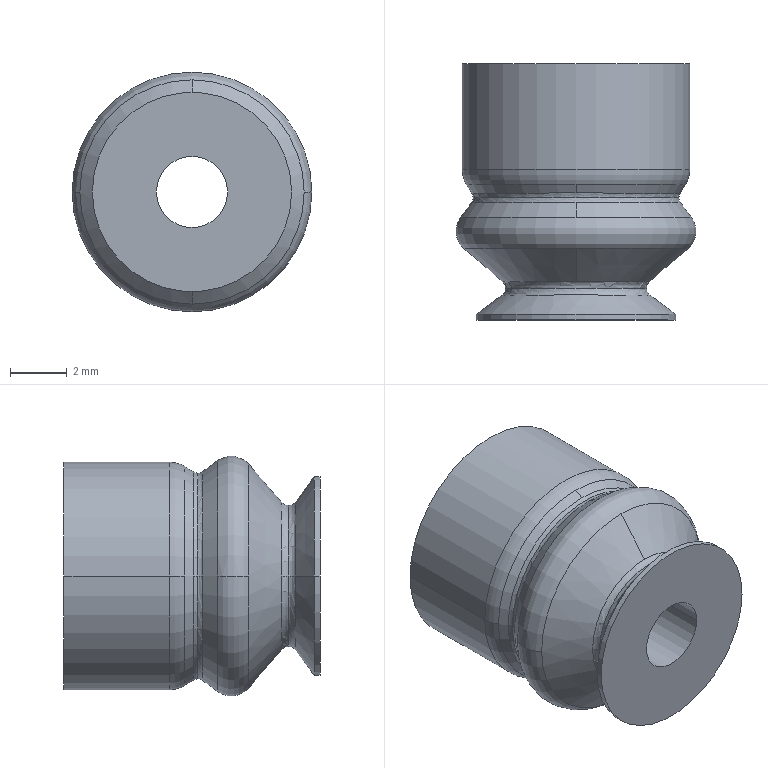Part | SolidWorks | features BaseBody 1 | 1 solid | 28 faces | box 8.435 x 9 x 8.435 mm | volume 355.359 mm3 | torus 12 | cone 8 | cylinder 6 | plane 2 | commonest cylinder face diameters 2.5 x2 7 x2 8 x2
STEP:
#1=CARTESIAN_POINT('',(-3.662,4.459,0.));
#2=VERTEX_POINT('',#1);
#3=CARTESIAN_POINT('',(-3.616,4.3,0.));
#4=VERTEX_POINT('',#3);
#5=CARTESIAN_POINT('',(-3.916,4.3,0.));
#6=DIRECTION('',(0.,0.,-1.));
#7=DIRECTION('',(0.,1.,0.));
#8=AXIS2_PLACEMENT_3D('',#5,#6,#7);
#9=CIRCLE('',#8,0.3);
#10=EDGE_CURVE('',#2,#4,#9,.T.);
#11=ORIENTED_EDGE('',*,*,#10,.T.);
#12=CARTESIAN_POINT('',(3.616,4.3,0.));
#13=VERTEX_POINT('',#12);
#14=CARTESIAN_POINT('',(0.,4.3,0.));
#15=DIRECTION('',(0.,1.,0.));
#16=DIRECTION('',(-1.,0.,0.));
#17=AXIS2_PLACEMENT_3D('',#14,#15,#16);
#18=CIRCLE('',#17,3.616);
#19=EDGE_CURVE('',#4,#13,#18,.T.);
#20=ORIENTED_EDGE('',*,*,#19,.T.);
#21=CARTESIAN_POINT('',(3.662,4.459,0.));
#22=VERTEX_POINT('',#21);
#23=CARTESIAN_POINT('',(3.916,4.3,0.));
#24=DIRECTION('',(0.,0.,1.));
#25=DIRECTION('',(1.,0.,0.));
#26=AXIS2_PLACEMENT_3D('',#23,#24,#25);
#27=CIRCLE('',#26,0.3);
#28=EDGE_CURVE('',#22,#13,#27,.T.);
#29=ORIENTED_EDGE('',*,*,#28,.F.);
#30=CARTESIAN_POINT('',(0.,4.459,3.662));
#31=VERTEX_POINT('',#30);
#32=CARTESIAN_POINT('',(0.,4.459,0.));
#33=DIRECTION('',(0.,1.,0.));
#34=DIRECTION('',(1.,0.,0.));
#35=AXIS2_PLACEMENT_3D('',#32,#33,#34);
#36=CIRCLE('',#35,3.662);
#37=EDGE_CURVE('',#31,#22,#36,.T.);
#38=ORIENTED_EDGE('',*,*,#37,.F.);
#39=CARTESIAN_POINT('',(0.,4.459,0.));
#40=DIRECTION('',(0.,1.,0.));
#41=DIRECTION('',(1.,0.,0.));
#42=AXIS2_PLACEMENT_3D('',#39,#40,#41);
#43=CIRCLE('',#42,3.662);
#44=EDGE_CURVE('',#2,#31,#43,.T.);
#45=ORIENTED_EDGE('',*,*,#44,.F.);
#46=EDGE_LOOP('',(#11,#20,#29,#38,#45));
#47=FACE_OUTER_BOUND('',#46,.T.);
#48=CARTESIAN_POINT('',(0.,4.3,0.));
#49=DIRECTION('',(0.,1.,0.));
#50=DIRECTION('',(-1.,0.,0.));
#51=AXIS2_PLACEMENT_3D('',#48,#49,#50);
#52=TOROIDAL_SURFACE('',#51,3.916,0.3);
#53=ADVANCED_FACE('',(#47),#52,.F.);
#54=CARTESIAN_POINT('',(-2.582,1.344,0.));
#55=VERTEX_POINT('',#54);
#56=CARTESIAN_POINT('',(-2.478,1.116,0.));
#57=VERTEX_POINT('',#56);
#58=CARTESIAN_POINT('',(-2.778,1.116,0.));
#59=DIRECTION('',(0.,0.,-1.));
#60=DIRECTION('',(-1.,0.,0.));
#61=AXIS2_PLACEMENT_3D('',#58,#59,#60);
#62=CIRCLE('',#61,0.3);
#63=EDGE_CURVE('',#55,#57,#62,.T.);
#64=ORIENTED_EDGE('',*,*,#63,.T.);
#65=CARTESIAN_POINT('',(2.478,1.116,0.));
#66=VERTEX_POINT('',#65);
#67=CARTESIAN_POINT('',(0.,1.116,0.));
#68=DIRECTION('',(0.,1.,0.));
#69=DIRECTION('',(-1.,0.,0.));
#70=AXIS2_PLACEMENT_3D('',#67,#68,#69);
#71=CIRCLE('',#70,2.478);
#72=EDGE_CURVE('',#57,#66,#71,.T.);
#73=ORIENTED_EDGE('',*,*,#72,.T.);
#74=CARTESIAN_POINT('',(2.582,1.344,0.));
#75=VERTEX_POINT('',#74);
#76=CARTESIAN_POINT('',(2.778,1.116,0.));
#77=DIRECTION('',(0.,0.,1.));
#78=DIRECTION('',(1.,0.,0.));
#79=AXIS2_PLACEMENT_3D('',#76,#77,#78);
#80=CIRCLE('',#79,0.3);
#81=EDGE_CURVE('',#75,#66,#80,.T.);
#82=ORIENTED_EDGE('',*,*,#81,.F.);
#83=CARTESIAN_POINT('',(0.,1.344,2.582));
#84=VERTEX_POINT('',#83);
#85=CARTESIAN_POINT('',(0.,1.344,0.));
#86=DIRECTION('',(0.,1.,0.));
#87=DIRECTION('',(0.,0.,1.));
#88=AXIS2_PLACEMENT_3D('',#85,#86,#87);
#89=CIRCLE('',#88,2.582);
#90=EDGE_CURVE('',#84,#75,#89,.T.);
#91=ORIENTED_EDGE('',*,*,#90,.F.);
#92=CARTESIAN_POINT('',(0.,1.344,0.));
#93=DIRECTION('',(0.,1.,0.));
#94=DIRECTION('',(0.,0.,1.));
#95=AXIS2_PLACEMENT_3D('',#92,#93,#94);
#96=CIRCLE('',#95,2.582);
#97=EDGE_CURVE('',#55,#84,#96,.T.);
#98=ORIENTED_EDGE('',*,*,#97,.F.);
#99=EDGE_LOOP('',(#64,#73,#82,#91,#98));
#100=FACE_OUTER_BOUND('',#99,.T.);
#101=CARTESIAN_POINT('',(0.,1.116,0.));
#102=DIRECTION('',(0.,1.,0.));
#103=DIRECTION('',(-1.,0.,0.));
#104=AXIS2_PLACEMENT_3D('',#101,#102,#103);
#105=TOROIDAL_SURFACE('',#104,2.778,0.3);
#106=ADVANCED_FACE('',(#100),#105,.F.);
#107=ORIENTED_EDGE('',*,*,#81,.T.);
#108=CARTESIAN_POINT('',(0.,1.116,0.));
#109=DIRECTION('',(0.,1.,0.));
#110=DIRECTION('',(-1.,0.,0.));
#111=AXIS2_PLACEMENT_3D('',#108,#109,#110);
#112=CIRCLE('',#111,2.478);
#113=EDGE_CURVE('',#66,#57,#112,.T.);
#114=ORIENTED_EDGE('',*,*,#113,.T.);
#115=ORIENTED_EDGE('',*,*,#63,.F.);
#116=CARTESIAN_POINT('',(0.,1.344,-2.582));
#117=VERTEX_POINT('',#116);
#118=CARTESIAN_POINT('',(0.,1.344,0.));
#119=DIRECTION('',(0.,1.,0.));
#120=DIRECTION('',(0.,0.,1.));
#121=AXIS2_PLACEMENT_3D('',#118,#119,#120);
#122=CIRCLE('',#121,2.582);
#123=EDGE_CURVE('',#117,#55,#122,.T.);
#124=ORIENTED_EDGE('',*,*,#123,.F.);
#125=CARTESIAN_POINT('',(0.,1.344,0.));
#126=DIRECTION('',(0.,1.,0.));
#127=DIRECTION('',(0.,0.,1.));
#128=AXIS2_PLACEMENT_3D('',#125,#126,#127);
#129=CIRCLE('',#128,2.582);
#130=EDGE_CURVE('',#75,#117,#129,.T.);
#131=ORIENTED_EDGE('',*,*,#130,.F.);
#132=EDGE_LOOP('',(#107,#114,#115,#124,#131));
#133=FACE_OUTER_BOUND('',#132,.T.);
#134=CARTESIAN_POINT('',(0.,1.116,0.));
#135=DIRECTION('',(0.,1.,0.));
#136=DIRECTION('',(-1.,0.,0.));
#137=AXIS2_PLACEMENT_3D('',#134,#135,#136);
#138=TOROIDAL_SURFACE('',#137,2.778,0.3);
#139=ADVANCED_FACE('',(#133),#138,.F.);
#140=ORIENTED_EDGE('',*,*,#28,.T.);
#141=CARTESIAN_POINT('',(0.,4.3,0.));
#142=DIRECTION('',(0.,1.,0.));
#143=DIRECTION('',(-1.,0.,0.));
#144=AXIS2_PLACEMENT_3D('',#141,#142,#143);
#145=CIRCLE('',#144,3.616);
#146=EDGE_CURVE('',#13,#4,#145,.T.);
#147=ORIENTED_EDGE('',*,*,#146,.T.);
#148=ORIENTED_EDGE('',*,*,#10,.F.);
#149=CARTESIAN_POINT('',(0.,4.459,-3.662));
#150=VERTEX_POINT('',#149);
#151=CARTESIAN_POINT('',(0.,4.459,0.));
#152=DIRECTION('',(0.,1.,0.));
#153=DIRECTION('',(1.,0.,0.));
#154=AXIS2_PLACEMENT_3D('',#151,#152,#153);
#155=CIRCLE('',#154,3.662);
#156=EDGE_CURVE('',#150,#2,#155,.T.);
#157=ORIENTED_EDGE('',*,*,#156,.F.);
#158=CARTESIAN_POINT('',(0.,4.459,0.));
#159=DIRECTION('',(0.,1.,0.));
#160=DIRECTION('',(1.,0.,0.));
#161=AXIS2_PLACEMENT_3D('',#158,#159,#160);
#162=CIRCLE('',#161,3.662);
#163=EDGE_CURVE('',#22,#150,#162,.T.);
#164=ORIENTED_EDGE('',*,*,#163,.F.);
#165=EDGE_LOOP('',(#140,#147,#148,#157,#164));
#166=FACE_OUTER_BOUND('',#165,.T.);
#167=CARTESIAN_POINT('',(0.,4.3,0.));
#168=DIRECTION('',(0.,1.,0.));
#169=DIRECTION('',(-1.,0.,0.));
#170=AXIS2_PLACEMENT_3D('',#167,#168,#169);
#171=TOROIDAL_SURFACE('',#170,3.916,0.3);
#172=ADVANCED_FACE('',(#166),#171,.F.);
#173=CARTESIAN_POINT('',(0.,4.757,3.848));
#174=VERTEX_POINT('',#173);
#175=CARTESIAN_POINT('',(3.848,4.757,0.));
#176=VERTEX_POINT('',#175);
#177=CARTESIAN_POINT('',(0.,4.757,0.));
#178=DIRECTION('',(0.,1.,0.));
#179=DIRECTION('',(0.,0.,1.));
#180=AXIS2_PLACEMENT_3D('',#177,#178,#179);
#181=CIRCLE('',#180,3.848);
#182=EDGE_CURVE('',#174,#176,#181,.T.);
#183=ORIENTED_EDGE('',*,*,#182,.T.);
#184=CARTESIAN_POINT('',(4.,5.287,0.));
#185=VERTEX_POINT('',#184);
#186=CARTESIAN_POINT('',(3.,5.287,0.));
#187=DIRECTION('',(0.,0.,1.));
#188=DIRECTION('',(1.,0.,0.));
#189=AXIS2_PLACEMENT_3D('',#186,#187,#188);
#190=CIRCLE('',#189,1.);
#191=EDGE_CURVE('',#176,#185,#190,.T.);
#192=ORIENTED_EDGE('',*,*,#191,.T.);
#193=CARTESIAN_POINT('',(-4.,5.287,0.));
#194=VERTEX_POINT('',#193);
#195=CARTESIAN_POINT('',(0.,5.287,0.));
#196=DIRECTION('',(0.,1.,0.));
#197=DIRECTION('',(1.,0.,0.));
#198=AXIS2_PLACEMENT_3D('',#195,#196,#197);
#199=CIRCLE('',#198,4.);
#200=EDGE_CURVE('',#194,#185,#199,.T.);
#201=ORIENTED_EDGE('',*,*,#200,.F.);
#202=CARTESIAN_POINT('',(-3.848,4.757,0.));
#203=VERTEX_POINT('',#202);
#204=CARTESIAN_POINT('',(-3.,5.287,0.));
#205=DIRECTION('',(0.,0.,-1.));
#206=DIRECTION('',(-1.,0.,0.));
#207=AXIS2_PLACEMENT_3D('',#204,#205,#206);
#208=CIRCLE('',#207,1.);
#209=EDGE_CURVE('',#203,#194,#208,.T.);
#210=ORIENTED_EDGE('',*,*,#209,.F.);
#211=CARTESIAN_POINT('',(0.,4.757,0.));
#212=DIRECTION('',(0.,1.,0.));
#213=DIRECTION('',(0.,0.,1.));
#214=AXIS2_PLACEMENT_3D('',#211,#212,#213);
#215=CIRCLE('',#214,3.848);
#216=EDGE_CURVE('',#203,#174,#215,.T.);
#217=ORIENTED_EDGE('',*,*,#216,.T.);
#218=EDGE_LOOP('',(#183,#192,#201,#210,#217));
#219=FACE_OUTER_BOUND('',#218,.T.);
#220=CARTESIAN_POINT('',(0.,5.287,0.));
#221=DIRECTION('',(0.,1.,0.));
#222=DIRECTION('',(-1.,0.,0.));
#223=AXIS2_PLACEMENT_3D('',#220,#221,#222);
#224=TOROIDAL_SURFACE('',#223,3.,1.);
#225=ADVANCED_FACE('',(#219),#224,.T.);
#226=ORIENTED_EDGE('',*,*,#146,.F.);
#227=CARTESIAN_POINT('',(3.675,4.122,0.));
#228=VERTEX_POINT('',#227);
#229=CARTESIAN_POINT('',(3.916,4.3,0.));
#230=DIRECTION('',(0.,0.,1.));
#231=DIRECTION('',(1.,0.,0.));
#232=AXIS2_PLACEMENT_3D('',#229,#230,#231);
#233=CIRCLE('',#232,0.3);
#234=EDGE_CURVE('',#13,#228,#233,.T.);
#235=ORIENTED_EDGE('',*,*,#234,.T.);
#236=CARTESIAN_POINT('',(0.,4.122,-3.675));
#237=VERTEX_POINT('',#236);
#238=CARTESIAN_POINT('',(0.,4.122,0.));
#239=DIRECTION('',(0.,-1.,0.));
#240=DIRECTION('',(0.,0.,1.));
#241=AXIS2_PLACEMENT_3D('',#238,#239,#240);
#242=CIRCLE('',#241,3.675);
#243=EDGE_CURVE('',#237,#228,#242,.T.);
#244=ORIENTED_EDGE('',*,*,#243,.F.);
#245=CARTESIAN_POINT('',(-3.675,4.122,0.));
#246=VERTEX_POINT('',#245);
#247=CARTESIAN_POINT('',(0.,4.122,0.));
#248=DIRECTION('',(0.,-1.,0.));
#249=DIRECTION('',(0.,0.,1.));
#250=AXIS2_PLACEMENT_3D('',#247,#248,#249);
#251=CIRCLE('',#250,3.675);
#252=EDGE_CURVE('',#246,#237,#251,.T.);
#253=ORIENTED_EDGE('',*,*,#252,.F.);
#254=CARTESIAN_POINT('',(-3.916,4.3,0.));
#255=DIRECTION('',(0.,0.,-1.));
#256=DIRECTION('',(0.,1.,0.));
#257=AXIS2_PLACEMENT_3D('',#254,#255,#256);
#258=CIRCLE('',#257,0.3);
#259=EDGE_CURVE('',#4,#246,#258,.T.);
#260=ORIENTED_EDGE('',*,*,#259,.F.);
#261=EDGE_LOOP('',(#226,#235,#244,#253,#260));
#262=FACE_OUTER_BOUND('',#261,.T.);
#263=CARTESIAN_POINT('',(0.,4.3,0.));
#264=DIRECTION('',(0.,1.,0.));
#265=DIRECTION('',(-1.,0.,0.));
#266=AXIS2_PLACEMENT_3D('',#263,#264,#265);
#267=TOROIDAL_SURFACE('',#266,3.916,0.3);
#268=ADVANCED_FACE('',(#262),#267,.F.);
#269=ORIENTED_EDGE('',*,*,#113,.F.);
#270=CARTESIAN_POINT('',(2.598,0.8765,0.));
#271=VERTEX_POINT('',#270);
#272=CARTESIAN_POINT('',(2.778,1.116,0.));
#273=DIRECTION('',(0.,0.,1.));
#274=DIRECTION('',(1.,0.,0.));
#275=AXIS2_PLACEMENT_3D('',#272,#273,#274);
#276=CIRCLE('',#275,0.3);
#277=EDGE_CURVE('',#66,#271,#276,.T.);
#278=ORIENTED_EDGE('',*,*,#277,.T.);
#279=CARTESIAN_POINT('',(-2.598,0.8765,0.));
#280=VERTEX_POINT('',#279);
#281=CARTESIAN_POINT('',(0.,0.8765,0.));
#282=DIRECTION('',(0.,-1.,0.));
#283=DIRECTION('',(1.,0.,0.));
#284=AXIS2_PLACEMENT_3D('',#281,#282,#283);
#285=CIRCLE('',#284,2.598);
#286=EDGE_CURVE('',#280,#271,#285,.T.);
#287=ORIENTED_EDGE('',*,*,#286,.F.);
#288=CARTESIAN_POINT('',(-2.778,1.116,0.));
#289=DIRECTION('',(0.,0.,-1.));
#290=DIRECTION('',(-1.,0.,0.));
#291=AXIS2_PLACEMENT_3D('',#288,#289,#290);
#292=CIRCLE('',#291,0.3);
#293=EDGE_CURVE('',#57,#280,#292,.T.);
#294=ORIENTED_EDGE('',*,*,#293,.F.);
#295=EDGE_LOOP('',(#269,#278,#287,#294));
#296=FACE_OUTER_BOUND('',#295,.T.);
#297=CARTESIAN_POINT('',(0.,1.116,0.));
#298=DIRECTION('',(0.,1.,0.));
#299=DIRECTION('',(-1.,0.,0.));
#300=AXIS2_PLACEMENT_3D('',#297,#298,#299);
#301=TOROIDAL_SURFACE('',#300,2.778,0.3);
#302=ADVANCED_FACE('',(#296),#301,.F.);
#303=CARTESIAN_POINT('',(0.,2.517,3.94));
#304=VERTEX_POINT('',#303);
#305=CARTESIAN_POINT('',(3.94,2.517,0.));
#306=VERTEX_POINT('',#305);
#307=CARTESIAN_POINT('',(0.,2.517,0.));
#308=DIRECTION('',(0.,1.,0.));
#309=DIRECTION('',(0.,0.,1.));
#310=AXIS2_PLACEMENT_3D('',#307,#308,#309);
#311=CIRCLE('',#310,3.94);
#312=EDGE_CURVE('',#304,#306,#311,.T.);
#313=ORIENTED_EDGE('',*,*,#312,.T.);
#314=CARTESIAN_POINT('',(4.062,3.596,0.));
#315=VERTEX_POINT('',#314);
#316=CARTESIAN_POINT('',(3.417,3.122,0.));
#317=DIRECTION('',(0.,0.,1.));
#318=DIRECTION('',(1.,0.,0.));
#319=AXIS2_PLACEMENT_3D('',#316,#317,#318);
#320=CIRCLE('',#319,0.8);
#321=EDGE_CURVE('',#306,#315,#320,.T.);
#322=ORIENTED_EDGE('',*,*,#321,.T.);
#323=CARTESIAN_POINT('',(0.,3.596,4.062));
#324=VERTEX_POINT('',#323);
#325=CARTESIAN_POINT('',(0.,3.596,0.));
#326=DIRECTION('',(0.,1.,0.));
#327=DIRECTION('',(1.,0.,0.));
#328=AXIS2_PLACEMENT_3D('',#325,#326,#327);
#329=CIRCLE('',#328,4.062);
#330=EDGE_CURVE('',#324,#315,#329,.T.);
#331=ORIENTED_EDGE('',*,*,#330,.F.);
#332=CARTESIAN_POINT('',(-4.062,3.596,0.));
#333=VERTEX_POINT('',#332);
#334=CARTESIAN_POINT('',(0.,3.596,0.));
#335=DIRECTION('',(0.,1.,0.));
#336=DIRECTION('',(1.,0.,0.));
#337=AXIS2_PLACEMENT_3D('',#334,#335,#336);
#338=CIRCLE('',#337,4.062);
#339=EDGE_CURVE('',#333,#324,#338,.T.);
#340=ORIENTED_EDGE('',*,*,#339,.F.);
#341=CARTESIAN_POINT('',(-3.94,2.517,0.));
#342=VERTEX_POINT('',#341);
#343=CARTESIAN_POINT('',(-3.417,3.122,0.));
#344=DIRECTION('',(0.,0.,-1.));
#345=DIRECTION('',(-1.,0.,0.));
#346=AXIS2_PLACEMENT_3D('',#343,#344,#345);
#347=CIRCLE('',#346,0.8);
#348=EDGE_CURVE('',#342,#333,#347,.T.);
#349=ORIENTED_EDGE('',*,*,#348,.F.);
#350=CARTESIAN_POINT('',(0.,2.517,0.));
#351=DIRECTION('',(0.,1.,0.));
#352=DIRECTION('',(0.,0.,1.));
#353=AXIS2_PLACEMENT_3D('',#350,#351,#352);
#354=CIRCLE('',#353,3.94);
#355=EDGE_CURVE('',#342,#304,#354,.T.);
#356=ORIENTED_EDGE('',*,*,#355,.T.);
#357=EDGE_LOOP('',(#313,#322,#331,#340,#349,#356));
#358=FACE_OUTER_BOUND('',#357,.T.);
#359=CARTESIAN_POINT('',(0.,3.122,0.));
#360=DIRECTION('',(0.,1.,0.));
#361=DIRECTION('',(-1.,0.,0.));
#362=AXIS2_PLACEMENT_3D('',#359,#360,#361);
#363=TOROIDAL_SURFACE('',#362,3.417,0.8);
#364=ADVANCED_FACE('',(#358),#363,.T.);
#365=CARTESIAN_POINT('',(4.,9.,0.));
#366=VERTEX_POINT('',#365);
#367=CARTESIAN_POINT('',(-4.,9.,0.));
#368=VERTEX_POINT('',#367);
#369=CARTESIAN_POINT('',(0.,9.,0.));
#370=DIRECTION('',(0.,-1.,0.));
#371=DIRECTION('',(1.,0.,0.));
#372=AXIS2_PLACEMENT_3D('',#369,#370,#371);
#373=CIRCLE('',#372,4.);
#374=EDGE_CURVE('',#366,#368,#373,.T.);
#375=ORIENTED_EDGE('',*,*,#374,.T.);
#376=CARTESIAN_POINT('',(-4.,7.143,0.));
#377=DIRECTION('',(0.,-1.,0.));
#378=VECTOR('',#377,1000.);
#379=LINE('',#376,#378);
#380=EDGE_CURVE('',#368,#194,#379,.T.);
#381=ORIENTED_EDGE('',*,*,#380,.T.);
#382=ORIENTED_EDGE('',*,*,#200,.T.);
#383=CARTESIAN_POINT('',(4.,7.143,0.));
#384=DIRECTION('',(0.,-1.,0.));
#385=VECTOR('',#384,1000.);
#386=LINE('',#383,#385);
#387=EDGE_CURVE('',#366,#185,#386,.T.);
#388=ORIENTED_EDGE('',*,*,#387,.F.);
#389=EDGE_LOOP('',(#375,#381,#382,#388));
#390=FACE_OUTER_BOUND('',#389,.T.);
#391=CARTESIAN_POINT('',(0.,7.143,0.));
#392=DIRECTION('',(0.,-1.,0.));
#393=DIRECTION('',(1.,0.,0.));
#394=AXIS2_PLACEMENT_3D('',#391,#392,#393);
#395=CYLINDRICAL_SURFACE('',#394,4.);
#396=ADVANCED_FACE('',(#390),#395,.T.);
#397=CARTESIAN_POINT('',(-1.25,9.,0.));
#398=VERTEX_POINT('',#397);
#399=CARTESIAN_POINT('',(1.25,9.,0.));
#400=VERTEX_POINT('',#399);
#401=CARTESIAN_POINT('',(0.,9.,0.));
#402=DIRECTION('',(0.,-1.,0.));
#403=DIRECTION('',(1.,0.,0.));
#404=AXIS2_PLACEMENT_3D('',#401,#402,#403);
#405=CIRCLE('',#404,1.25);
#406=EDGE_CURVE('',#398,#400,#405,.T.);
#407=ORIENTED_EDGE('',*,*,#406,.F.);
#408=CARTESIAN_POINT('',(-1.25,0.,0.));
#409=VERTEX_POINT('',#408);
#410=CARTESIAN_POINT('',(-1.25,4.5,0.));
#411=DIRECTION('',(0.,-1.,0.));
#412=VECTOR('',#411,1000.);
#413=LINE('',#410,#412);
#414=EDGE_CURVE('',#398,#409,#413,.T.);
#415=ORIENTED_EDGE('',*,*,#414,.T.);
#416=CARTESIAN_POINT('',(1.25,0.,0.));
#417=VERTEX_POINT('',#416);
#418=CARTESIAN_POINT('',(0.,0.,0.));
#419=DIRECTION('',(0.,1.,0.));
#420=DIRECTION('',(1.,0.,0.));
#421=AXIS2_PLACEMENT_3D('',#418,#419,#420);
#422=CIRCLE('',#421,1.25);
#423=EDGE_CURVE('',#417,#409,#422,.T.);
#424=ORIENTED_EDGE('',*,*,#423,.F.);
#425=CARTESIAN_POINT('',(1.25,4.5,0.));
#426=DIRECTION('',(0.,-1.,0.));
#427=VECTOR('',#426,1000.);
#428=LINE('',#425,#427);
#429=EDGE_CURVE('',#400,#417,#428,.T.);
#430=ORIENTED_EDGE('',*,*,#429,.F.);
#431=EDGE_LOOP('',(#407,#415,#424,#430));
#432=FACE_OUTER_BOUND('',#431,.T.);
#433=CARTESIAN_POINT('',(0.,4.5,0.));
#434=DIRECTION('',(0.,-1.,0.));
#435=DIRECTION('',(1.,0.,0.));
#436=AXIS2_PLACEMENT_3D('',#433,#434,#435);
#437=CYLINDRICAL_SURFACE('',#436,1.25);
#438=ADVANCED_FACE('',(#432),#437,.F.);
#439=ORIENTED_EDGE('',*,*,#37,.T.);
#440=ORIENTED_EDGE('',*,*,#163,.T.);
#441=CARTESIAN_POINT('',(0.,4.757,-3.848));
#442=VERTEX_POINT('',#441);
#443=CARTESIAN_POINT('',(0.,4.757,-3.848));
#444=DIRECTION('',(0.,0.848,-0.53));
#445=VECTOR('',#444,1000.);
#446=LINE('',#443,#445);
#447=EDGE_CURVE('',#150,#442,#446,.T.);
#448=ORIENTED_EDGE('',*,*,#447,.T.);
#449=CARTESIAN_POINT('',(0.,4.757,0.));
#450=DIRECTION('',(0.,1.,0.));
#451=DIRECTION('',(0.,0.,1.));
#452=AXIS2_PLACEMENT_3D('',#449,#450,#451);
#453=CIRCLE('',#452,3.848);
#454=EDGE_CURVE('',#176,#442,#453,.T.);
#455=ORIENTED_EDGE('',*,*,#454,.F.);
#456=ORIENTED_EDGE('',*,*,#182,.F.);
#457=CARTESIAN_POINT('',(0.,4.757,3.848));
#458=DIRECTION('',(0.,0.848,0.53));
#459=VECTOR('',#458,1000.);
#460=LINE('',#457,#459);
#461=EDGE_CURVE('',#31,#174,#460,.T.);
#462=ORIENTED_EDGE('',*,*,#461,.F.);
#463=EDGE_LOOP('',(#439,#440,#448,#455,#456,#462));
#464=FACE_OUTER_BOUND('',#463,.T.);
#465=CARTESIAN_POINT('',(0.,4.757,0.));
#466=DIRECTION('',(0.,1.,0.));
#467=DIRECTION('',(0.,0.,1.));
#468=AXIS2_PLACEMENT_3D('',#465,#466,#467);
#469=CONICAL_SURFACE('',#468,3.848,0.5586);
#470=ADVANCED_FACE('',(#464),#469,.T.);
#471=CARTESIAN_POINT('',(3.5,0.2,0.));
#472=VERTEX_POINT('',#471);
#473=CARTESIAN_POINT('',(-3.5,0.2,0.));
#474=VERTEX_POINT('',#473);
#475=CARTESIAN_POINT('',(0.,0.2,0.));
#476=DIRECTION('',(0.,-1.,0.));
#477=DIRECTION('',(1.,0.,0.));
#478=AXIS2_PLACEMENT_3D('',#475,#476,#477);
#479=CIRCLE('',#478,3.5);
#480=EDGE_CURVE('',#472,#474,#479,.T.);
#481=ORIENTED_EDGE('',*,*,#480,.T.);
#482=CARTESIAN_POINT('',(-3.5,0.,0.));
#483=VERTEX_POINT('',#482);
#484=CARTESIAN_POINT('',(-3.5,0.1,0.));
#485=DIRECTION('',(0.,-1.,0.));
#486=VECTOR('',#485,1000.);
#487=LINE('',#484,#486);
#488=EDGE_CURVE('',#474,#483,#487,.T.);
#489=ORIENTED_EDGE('',*,*,#488,.T.);
#490=CARTESIAN_POINT('',(3.5,0.,0.));
#491=VERTEX_POINT('',#490);
#492=CARTESIAN_POINT('',(0.,0.,0.));
#493=DIRECTION('',(0.,-1.,0.));
#494=DIRECTION('',(1.,0.,0.));
#495=AXIS2_PLACEMENT_3D('',#492,#493,#494);
#496=CIRCLE('',#495,3.5);
#497=EDGE_CURVE('',#491,#483,#496,.T.);
#498=ORIENTED_EDGE('',*,*,#497,.F.);
#499=CARTESIAN_POINT('',(3.5,0.1,0.));
#500=DIRECTION('',(0.,-1.,0.));
#501=VECTOR('',#500,1000.);
#502=LINE('',#499,#501);
#503=EDGE_CURVE('',#472,#491,#502,.T.);
#504=ORIENTED_EDGE('',*,*,#503,.F.);
#505=EDGE_LOOP('',(#481,#489,#498,#504));
#506=FACE_OUTER_BOUND('',#505,.T.);
#507=CARTESIAN_POINT('',(0.,0.1,0.));
#508=DIRECTION('',(0.,-1.,0.));
#509=DIRECTION('',(1.,0.,0.));
#510=AXIS2_PLACEMENT_3D('',#507,#508,#509);
#511=CYLINDRICAL_SURFACE('',#510,3.5);
#512=ADVANCED_FACE('',(#506),#511,.T.);
#513=CARTESIAN_POINT('',(0.,0.8765,0.));
#514=DIRECTION('',(0.,-1.,0.));
#515=DIRECTION('',(1.,0.,0.));
#516=AXIS2_PLACEMENT_3D('',#513,#514,#515);
#517=CIRCLE('',#516,2.598);
#518=EDGE_CURVE('',#271,#280,#517,.T.);
#519=ORIENTED_EDGE('',*,*,#518,.T.);
#520=CARTESIAN_POINT('',(-3.5,0.2,0.));
#521=DIRECTION('',(-0.8,-0.6,0.));
#522=VECTOR('',#521,1000.);
#523=LINE('',#520,#522);
#524=EDGE_CURVE('',#280,#474,#523,.T.);
#525=ORIENTED_EDGE('',*,*,#524,.T.);
#526=ORIENTED_EDGE('',*,*,#480,.F.);
#527=CARTESIAN_POINT('',(3.5,0.2,0.));
#528=DIRECTION('',(0.8,-0.6,0.));
#529=VECTOR('',#528,1000.);
#530=LINE('',#527,#529);
#531=EDGE_CURVE('',#271,#472,#530,.T.);
#532=ORIENTED_EDGE('',*,*,#531,.F.);
#533=EDGE_LOOP('',(#519,#525,#526,#532));
#534=FACE_OUTER_BOUND('',#533,.T.);
#535=CARTESIAN_POINT('',(0.,0.2,0.));
#536=DIRECTION('',(0.,-1.,0.));
#537=DIRECTION('',(1.,0.,0.));
#538=AXIS2_PLACEMENT_3D('',#535,#536,#537);
#539=CONICAL_SURFACE('',#538,3.5,0.9273);
#540=ADVANCED_FACE('',(#534),#539,.T.);
#541=ORIENTED_EDGE('',*,*,#243,.T.);
#542=CARTESIAN_POINT('',(0.,4.122,3.675));
#543=VERTEX_POINT('',#542);
#544=CARTESIAN_POINT('',(0.,4.122,0.));
#545=DIRECTION('',(0.,-1.,0.));
#546=DIRECTION('',(0.,0.,1.));
#547=AXIS2_PLACEMENT_3D('',#544,#545,#546);
#548=CIRCLE('',#547,3.675);
#549=EDGE_CURVE('',#228,#543,#548,.T.);
#550=ORIENTED_EDGE('',*,*,#549,.T.);
#551=CARTESIAN_POINT('',(0.,3.596,4.062));
#552=DIRECTION('',(0.,-0.8057,0.5924));
#553=VECTOR('',#552,1000.);
#554=LINE('',#551,#553);
#555=EDGE_CURVE('',#543,#324,#554,.T.);
#556=ORIENTED_EDGE('',*,*,#555,.T.);
#557=ORIENTED_EDGE('',*,*,#330,.T.);
#558=CARTESIAN_POINT('',(0.,3.596,-4.062));
#559=VERTEX_POINT('',#558);
#560=CARTESIAN_POINT('',(0.,3.596,0.));
#561=DIRECTION('',(0.,1.,0.));
#562=DIRECTION('',(1.,0.,0.));
#563=AXIS2_PLACEMENT_3D('',#560,#561,#562);
#564=CIRCLE('',#563,4.062);
#565=EDGE_CURVE('',#315,#559,#564,.T.);
#566=ORIENTED_EDGE('',*,*,#565,.T.);
#567=CARTESIAN_POINT('',(0.,3.596,-4.062));
#568=DIRECTION('',(0.,-0.8057,-0.5924));
#569=VECTOR('',#568,1000.);
#570=LINE('',#567,#569);
#571=EDGE_CURVE('',#237,#559,#570,.T.);
#572=ORIENTED_EDGE('',*,*,#571,.F.);
#573=EDGE_LOOP('',(#541,#550,#556,#557,#566,#572));
#574=FACE_OUTER_BOUND('',#573,.T.);
#575=CARTESIAN_POINT('',(0.,3.596,0.));
#576=DIRECTION('',(0.,-1.,0.));
#577=DIRECTION('',(0.,0.,-1.));
#578=AXIS2_PLACEMENT_3D('',#575,#576,#577);
#579=CONICAL_SURFACE('',#578,4.062,0.634);
#580=ADVANCED_FACE('',(#574),#579,.T.);
#581=ORIENTED_EDGE('',*,*,#90,.T.);
#582=ORIENTED_EDGE('',*,*,#130,.T.);
#583=CARTESIAN_POINT('',(0.,2.517,-3.94));
#584=VERTEX_POINT('',#583);
#585=CARTESIAN_POINT('',(0.,2.517,-3.94));
#586=DIRECTION('',(0.,0.6536,-0.7568));
#587=VECTOR('',#586,1000.);
#588=LINE('',#585,#587);
#589=EDGE_CURVE('',#117,#584,#588,.T.);
#590=ORIENTED_EDGE('',*,*,#589,.T.);
#591=CARTESIAN_POINT('',(0.,2.517,0.));
#592=DIRECTION('',(0.,1.,0.));
#593=DIRECTION('',(0.,0.,1.));
#594=AXIS2_PLACEMENT_3D('',#591,#592,#593);
#595=CIRCLE('',#594,3.94);
#596=EDGE_CURVE('',#306,#584,#595,.T.);
#597=ORIENTED_EDGE('',*,*,#596,.F.);
#598=ORIENTED_EDGE('',*,*,#312,.F.);
#599=CARTESIAN_POINT('',(0.,2.517,3.94));
#600=DIRECTION('',(0.,0.6536,0.7568));
#601=VECTOR('',#600,1000.);
#602=LINE('',#599,#601);
#603=EDGE_CURVE('',#84,#304,#602,.T.);
#604=ORIENTED_EDGE('',*,*,#603,.F.);
#605=EDGE_LOOP('',(#581,#582,#590,#597,#598,#604));
#606=FACE_OUTER_BOUND('',#605,.T.);
#607=CARTESIAN_POINT('',(0.,2.517,0.));
#608=DIRECTION('',(0.,1.,0.));
#609=DIRECTION('',(0.,0.,1.));
#610=AXIS2_PLACEMENT_3D('',#607,#608,#609);
#611=CONICAL_SURFACE('',#610,3.94,0.8584);
#612=ADVANCED_FACE('',(#606),#611,.T.);
#613=ORIENTED_EDGE('',*,*,#423,.T.);
#614=CARTESIAN_POINT('',(0.,0.,0.));
#615=DIRECTION('',(0.,1.,0.));
#616=DIRECTION('',(1.,0.,0.));
#617=AXIS2_PLACEMENT_3D('',#614,#615,#616);
#618=CIRCLE('',#617,1.25);
#619=EDGE_CURVE('',#409,#417,#618,.T.);
#620=ORIENTED_EDGE('',*,*,#619,.T.);
#621=EDGE_LOOP('',(#613,#620));
#622=FACE_BOUND('',#621,.T.);
#623=ORIENTED_EDGE('',*,*,#497,.T.);
#624=CARTESIAN_POINT('',(0.,0.,0.));
#625=DIRECTION('',(0.,-1.,0.));
#626=DIRECTION('',(1.,0.,0.));
#627=AXIS2_PLACEMENT_3D('',#624,#625,#626);
#628=CIRCLE('',#627,3.5);
#629=EDGE_CURVE('',#483,#491,#628,.T.);
#630=ORIENTED_EDGE('',*,*,#629,.T.);
#631=EDGE_LOOP('',(#623,#630));
#632=FACE_OUTER_BOUND('',#631,.T.);
#633=CARTESIAN_POINT('',(2.375,0.,0.));
#634=DIRECTION('',(0.,-1.,0.));
#635=DIRECTION('',(-1.,0.,0.));
#636=AXIS2_PLACEMENT_3D('',#633,#634,#635);
#637=PLANE('',#636);
#638=ADVANCED_FACE('',(#622,#632),#637,.T.);
#639=CARTESIAN_POINT('',(0.,9.,0.));
#640=DIRECTION('',(0.,-1.,0.));
#641=DIRECTION('',(1.,0.,0.));
#642=AXIS2_PLACEMENT_3D('',#639,#640,#641);
#643=CIRCLE('',#642,1.25);
#644=EDGE_CURVE('',#400,#398,#643,.T.);
#645=ORIENTED_EDGE('',*,*,#644,.T.);
#646=ORIENTED_EDGE('',*,*,#406,.T.);
#647=EDGE_LOOP('',(#645,#646));
#648=FACE_BOUND('',#647,.T.);
#649=ORIENTED_EDGE('',*,*,#374,.F.);
#650=CARTESIAN_POINT('',(0.,9.,0.));
#651=DIRECTION('',(0.,-1.,0.));
#652=DIRECTION('',(1.,0.,0.));
#653=AXIS2_PLACEMENT_3D('',#650,#651,#652);
#654=CIRCLE('',#653,4.);
#655=EDGE_CURVE('',#368,#366,#654,.T.);
#656=ORIENTED_EDGE('',*,*,#655,.F.);
#657=EDGE_LOOP('',(#649,#656));
#658=FACE_OUTER_BOUND('',#657,.T.);
#659=CARTESIAN_POINT('',(2.625,9.,0.));
#660=DIRECTION('',(0.,1.,0.));
#661=DIRECTION('',(0.,0.,-1.));
#662=AXIS2_PLACEMENT_3D('',#659,#660,#661);
#663=PLANE('',#662);
#664=ADVANCED_FACE('',(#648,#658),#663,.T.);
#665=ORIENTED_EDGE('',*,*,#589,.F.);
#666=ORIENTED_EDGE('',*,*,#123,.T.);
#667=ORIENTED_EDGE('',*,*,#97,.T.);
#668=ORIENTED_EDGE('',*,*,#603,.T.);
#669=ORIENTED_EDGE('',*,*,#355,.F.);
#670=CARTESIAN_POINT('',(0.,2.517,0.));
#671=DIRECTION('',(0.,1.,0.));
#672=DIRECTION('',(0.,0.,1.));
#673=AXIS2_PLACEMENT_3D('',#670,#671,#672);
#674=CIRCLE('',#673,3.94);
#675=EDGE_CURVE('',#584,#342,#674,.T.);
#676=ORIENTED_EDGE('',*,*,#675,.F.);
#677=EDGE_LOOP('',(#665,#666,#667,#668,#669,#676));
#678=FACE_OUTER_BOUND('',#677,.T.);
#679=CARTESIAN_POINT('',(0.,2.517,0.));
#680=DIRECTION('',(0.,1.,0.));
#681=DIRECTION('',(0.,0.,1.));
#682=AXIS2_PLACEMENT_3D('',#679,#680,#681);
#683=CONICAL_SURFACE('',#682,3.94,0.8584);
#684=ADVANCED_FACE('',(#678),#683,.T.);
#685=ORIENTED_EDGE('',*,*,#555,.F.);
#686=CARTESIAN_POINT('',(0.,4.122,0.));
#687=DIRECTION('',(0.,-1.,0.));
#688=DIRECTION('',(0.,0.,1.));
#689=AXIS2_PLACEMENT_3D('',#686,#687,#688);
#690=CIRCLE('',#689,3.675);
#691=EDGE_CURVE('',#543,#246,#690,.T.);
#692=ORIENTED_EDGE('',*,*,#691,.T.);
#693=ORIENTED_EDGE('',*,*,#252,.T.);
#694=ORIENTED_EDGE('',*,*,#571,.T.);
#695=CARTESIAN_POINT('',(0.,3.596,0.));
#696=DIRECTION('',(0.,1.,0.));
#697=DIRECTION('',(1.,0.,0.));
#698=AXIS2_PLACEMENT_3D('',#695,#696,#697);
#699=CIRCLE('',#698,4.062);
#700=EDGE_CURVE('',#559,#333,#699,.T.);
#701=ORIENTED_EDGE('',*,*,#700,.T.);
#702=ORIENTED_EDGE('',*,*,#339,.T.);
#703=EDGE_LOOP('',(#685,#692,#693,#694,#701,#702));
#704=FACE_OUTER_BOUND('',#703,.T.);
#705=CARTESIAN_POINT('',(0.,3.596,0.));
#706=DIRECTION('',(0.,-1.,0.));
#707=DIRECTION('',(0.,0.,-1.));
#708=AXIS2_PLACEMENT_3D('',#705,#706,#707);
#709=CONICAL_SURFACE('',#708,4.062,0.634);
#710=ADVANCED_FACE('',(#704),#709,.T.);
#711=ORIENTED_EDGE('',*,*,#524,.F.);
#712=ORIENTED_EDGE('',*,*,#286,.T.);
#713=ORIENTED_EDGE('',*,*,#531,.T.);
#714=CARTESIAN_POINT('',(0.,0.2,0.));
#715=DIRECTION('',(0.,-1.,0.));
#716=DIRECTION('',(1.,0.,0.));
#717=AXIS2_PLACEMENT_3D('',#714,#715,#716);
#718=CIRCLE('',#717,3.5);
#719=EDGE_CURVE('',#474,#472,#718,.T.);
#720=ORIENTED_EDGE('',*,*,#719,.F.);
#721=EDGE_LOOP('',(#711,#712,#713,#720));
#722=FACE_OUTER_BOUND('',#721,.T.);
#723=CARTESIAN_POINT('',(0.,0.2,0.));
#724=DIRECTION('',(0.,-1.,0.));
#725=DIRECTION('',(1.,0.,0.));
#726=AXIS2_PLACEMENT_3D('',#723,#724,#725);
#727=CONICAL_SURFACE('',#726,3.5,0.9273);
#728=ADVANCED_FACE('',(#722),#727,.T.);
#729=ORIENTED_EDGE('',*,*,#488,.F.);
#730=ORIENTED_EDGE('',*,*,#719,.T.);
#731=ORIENTED_EDGE('',*,*,#503,.T.);
#732=ORIENTED_EDGE('',*,*,#629,.F.);
#733=EDGE_LOOP('',(#729,#730,#731,#732));
#734=FACE_OUTER_BOUND('',#733,.T.);
#735=CARTESIAN_POINT('',(0.,0.1,0.));
#736=DIRECTION('',(0.,-1.,0.));
#737=DIRECTION('',(1.,0.,0.));
#738=AXIS2_PLACEMENT_3D('',#735,#736,#737);
#739=CYLINDRICAL_SURFACE('',#738,3.5);
#740=ADVANCED_FACE('',(#734),#739,.T.);
#741=ORIENTED_EDGE('',*,*,#447,.F.);
#742=ORIENTED_EDGE('',*,*,#156,.T.);
#743=ORIENTED_EDGE('',*,*,#44,.T.);
#744=ORIENTED_EDGE('',*,*,#461,.T.);
#745=ORIENTED_EDGE('',*,*,#216,.F.);
#746=CARTESIAN_POINT('',(0.,4.757,0.));
#747=DIRECTION('',(0.,1.,0.));
#748=DIRECTION('',(0.,0.,1.));
#749=AXIS2_PLACEMENT_3D('',#746,#747,#748);
#750=CIRCLE('',#749,3.848);
#751=EDGE_CURVE('',#442,#203,#750,.T.);
#752=ORIENTED_EDGE('',*,*,#751,.F.);
#753=EDGE_LOOP('',(#741,#742,#743,#744,#745,#752));
#754=FACE_OUTER_BOUND('',#753,.T.);
#755=CARTESIAN_POINT('',(0.,4.757,0.));
#756=DIRECTION('',(0.,1.,0.));
#757=DIRECTION('',(0.,0.,1.));
#758=AXIS2_PLACEMENT_3D('',#755,#756,#757);
#759=CONICAL_SURFACE('',#758,3.848,0.5586);
#760=ADVANCED_FACE('',(#754),#759,.T.);
#761=ORIENTED_EDGE('',*,*,#414,.F.);
#762=ORIENTED_EDGE('',*,*,#644,.F.);
#763=ORIENTED_EDGE('',*,*,#429,.T.);
#764=ORIENTED_EDGE('',*,*,#619,.F.);
#765=EDGE_LOOP('',(#761,#762,#763,#764));
#766=FACE_OUTER_BOUND('',#765,.T.);
#767=CARTESIAN_POINT('',(0.,4.5,0.));
#768=DIRECTION('',(0.,-1.,0.));
#769=DIRECTION('',(1.,0.,0.));
#770=AXIS2_PLACEMENT_3D('',#767,#768,#769);
#771=CYLINDRICAL_SURFACE('',#770,1.25);
#772=ADVANCED_FACE('',(#766),#771,.F.);
#773=ORIENTED_EDGE('',*,*,#380,.F.);
#774=ORIENTED_EDGE('',*,*,#655,.T.);
#775=ORIENTED_EDGE('',*,*,#387,.T.);
#776=CARTESIAN_POINT('',(0.,5.287,0.));
#777=DIRECTION('',(0.,1.,0.));
#778=DIRECTION('',(1.,0.,0.));
#779=AXIS2_PLACEMENT_3D('',#776,#777,#778);
#780=CIRCLE('',#779,4.);
#781=EDGE_CURVE('',#185,#194,#780,.T.);
#782=ORIENTED_EDGE('',*,*,#781,.T.);
#783=EDGE_LOOP('',(#773,#774,#775,#782));
#784=FACE_OUTER_BOUND('',#783,.T.);
#785=CARTESIAN_POINT('',(0.,7.143,0.));
#786=DIRECTION('',(0.,-1.,0.));
#787=DIRECTION('',(1.,0.,0.));
#788=AXIS2_PLACEMENT_3D('',#785,#786,#787);
#789=CYLINDRICAL_SURFACE('',#788,4.);
#790=ADVANCED_FACE('',(#784),#789,.T.);
#791=ORIENTED_EDGE('',*,*,#321,.F.);
#792=ORIENTED_EDGE('',*,*,#596,.T.);
#793=ORIENTED_EDGE('',*,*,#675,.T.);
#794=ORIENTED_EDGE('',*,*,#348,.T.);
#795=ORIENTED_EDGE('',*,*,#700,.F.);
#796=ORIENTED_EDGE('',*,*,#565,.F.);
#797=EDGE_LOOP('',(#791,#792,#793,#794,#795,#796));
#798=FACE_OUTER_BOUND('',#797,.T.);
#799=CARTESIAN_POINT('',(0.,3.122,0.));
#800=DIRECTION('',(0.,1.,0.));
#801=DIRECTION('',(-1.,0.,0.));
#802=AXIS2_PLACEMENT_3D('',#799,#800,#801);
#803=TOROIDAL_SURFACE('',#802,3.417,0.8);
#804=ADVANCED_FACE('',(#798),#803,.T.);
#805=ORIENTED_EDGE('',*,*,#72,.F.);
#806=ORIENTED_EDGE('',*,*,#293,.T.);
#807=ORIENTED_EDGE('',*,*,#518,.F.);
#808=ORIENTED_EDGE('',*,*,#277,.F.);
#809=EDGE_LOOP('',(#805,#806,#807,#808));
#810=FACE_OUTER_BOUND('',#809,.T.);
#811=CARTESIAN_POINT('',(0.,1.116,0.));
#812=DIRECTION('',(0.,1.,0.));
#813=DIRECTION('',(-1.,0.,0.));
#814=AXIS2_PLACEMENT_3D('',#811,#812,#813);
#815=TOROIDAL_SURFACE('',#814,2.778,0.3);
#816=ADVANCED_FACE('',(#810),#815,.F.);
#817=ORIENTED_EDGE('',*,*,#19,.F.);
#818=ORIENTED_EDGE('',*,*,#259,.T.);
#819=ORIENTED_EDGE('',*,*,#691,.F.);
#820=ORIENTED_EDGE('',*,*,#549,.F.);
#821=ORIENTED_EDGE('',*,*,#234,.F.);
#822=EDGE_LOOP('',(#817,#818,#819,#820,#821));
#823=FACE_OUTER_BOUND('',#822,.T.);
#824=CARTESIAN_POINT('',(0.,4.3,0.));
#825=DIRECTION('',(0.,1.,0.));
#826=DIRECTION('',(-1.,0.,0.));
#827=AXIS2_PLACEMENT_3D('',#824,#825,#826);
#828=TOROIDAL_SURFACE('',#827,3.916,0.3);
#829=ADVANCED_FACE('',(#823),#828,.F.);
#830=ORIENTED_EDGE('',*,*,#191,.F.);
#831=ORIENTED_EDGE('',*,*,#454,.T.);
#832=ORIENTED_EDGE('',*,*,#751,.T.);
#833=ORIENTED_EDGE('',*,*,#209,.T.);
#834=ORIENTED_EDGE('',*,*,#781,.F.);
#835=EDGE_LOOP('',(#830,#831,#832,#833,#834));
#836=FACE_OUTER_BOUND('',#835,.T.);
#837=CARTESIAN_POINT('',(0.,5.287,0.));
#838=DIRECTION('',(0.,1.,0.));
#839=DIRECTION('',(-1.,0.,0.));
#840=AXIS2_PLACEMENT_3D('',#837,#838,#839);
#841=TOROIDAL_SURFACE('',#840,3.,1.);
#842=ADVANCED_FACE('',(#836),#841,.T.);
#843=CLOSED_SHELL('',(#53,#106,#139,#172,#225,#268,#302,#364,#396,#438,#470,#512,#540,#580,#612,#638,#664,#684,#710,#728,#740,#760,#772,#790,#804,#816,#829,#842));
#844=MANIFOLD_SOLID_BREP('',#843);
#845=CARTESIAN_POINT('',(0.,0.,0.));
#846=DIRECTION('',(0.,0.,1.));
#847=DIRECTION('',(1.,0.,0.));
#848=AXIS2_PLACEMENT_3D('',#845,#846,#847);
#849=(LENGTH_UNIT()NAMED_UNIT(*)SI_UNIT(.MILLI.,.METRE.));
#850=UNCERTAINTY_MEASURE_WITH_UNIT(LENGTH_MEASURE(0.00001),#849,'','');
#851=(NAMED_UNIT(*)PLANE_ANGLE_UNIT()SI_UNIT($,.RADIAN.));
#852=(NAMED_UNIT(*)SI_UNIT($,.STERADIAN.)SOLID_ANGLE_UNIT());
#853=(GEOMETRIC_REPRESENTATION_CONTEXT(3)GLOBAL_UNCERTAINTY_ASSIGNED_CONTEXT((#850))GLOBAL_UNIT_ASSIGNED_CONTEXT((#849,#851,#852))REPRESENTATION_CONTEXT('',''));
#854=ADVANCED_BREP_SHAPE_REPRESENTATION('',(#844,#848),#853);